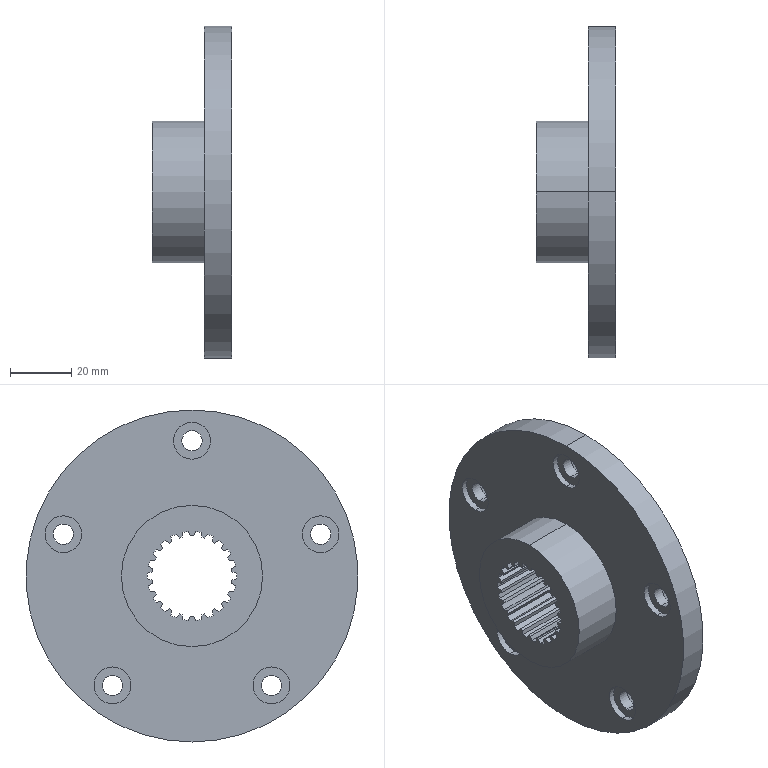Part | STEP file | Previa 01.sldasm-Part-5_Valor predeterminado | 1 solid | 135 faces | box 26 x 108 x 108 mm | volume 90690 mm3 | plane 75 | cylinder 46 | cone 10 | torus 4 | commonest cylinder face diameters 29 x22 6.6 x10 12 x10 46 x2 108 x2